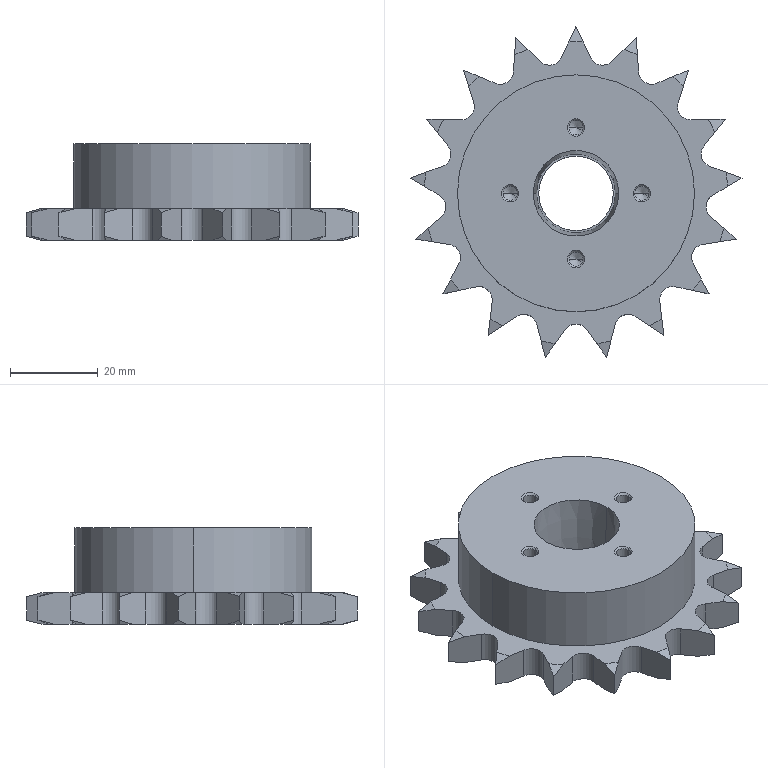Part | STEP file | LFSP40B17_17_Asp | 1 solid | 124 faces | box 75.676 x 75.353 x 22 mm | volume 51808 mm3 | cone 52 | plane 38 | cylinder 34 | commonest cylinder face diameters 6 x22 3.242 x8 17 x2 54 x2